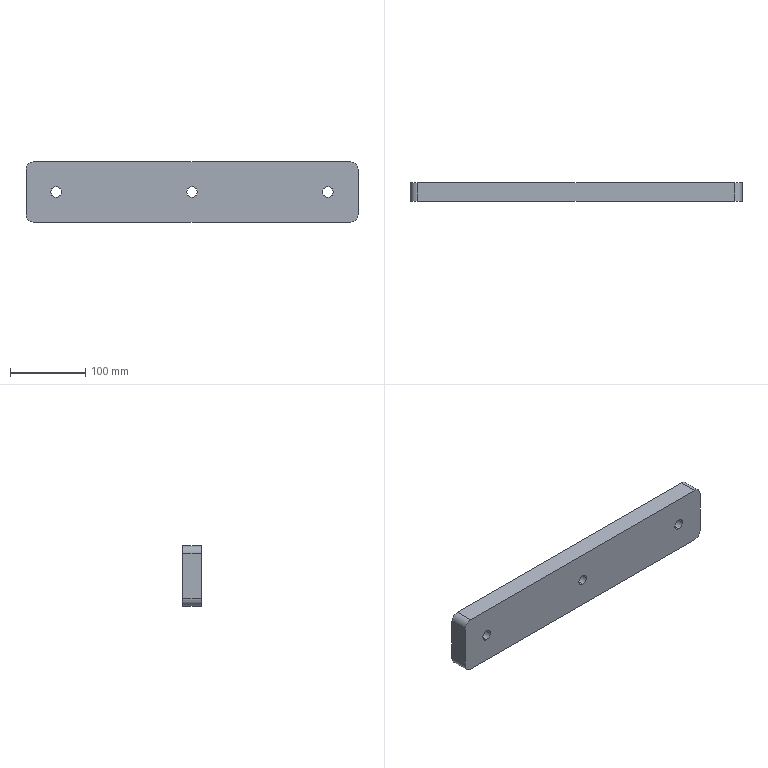Part | SolidWorks | features Fillet 1, FlatPattern 1, HoleWzd 1, LPattern 1, SMBaseFlange 1, SheetMetal 1 | 1 solid | 16 faces | box 440 x 25 x 80 mm | volume 866309 mm3 | cylinder 10 | plane 6 | commonest cylinder face diameters 14 x6 20 x4
STEP:
#1=CARTESIAN_POINT('',(180.,-25.,7.));
#2=VERTEX_POINT('',#1);
#3=CARTESIAN_POINT('',(180.,-25.,-7.));
#4=VERTEX_POINT('',#3);
#5=CARTESIAN_POINT('',(180.,-25.,0.));
#6=DIRECTION('',(0.,-1.,0.));
#7=DIRECTION('',(0.,0.,-1.));
#8=AXIS2_PLACEMENT_3D('',#5,#6,#7);
#9=CIRCLE('',#8,7.);
#10=EDGE_CURVE('',#2,#4,#9,.T.);
#11=ORIENTED_EDGE('',*,*,#10,.T.);
#12=CARTESIAN_POINT('',(180.,0.,-7.));
#13=VERTEX_POINT('',#12);
#14=CARTESIAN_POINT('',(180.,0.,-7.));
#15=DIRECTION('',(0.,1.,0.));
#16=VECTOR('',#15,1000.);
#17=LINE('',#14,#16);
#18=EDGE_CURVE('',#4,#13,#17,.T.);
#19=ORIENTED_EDGE('',*,*,#18,.T.);
#20=CARTESIAN_POINT('',(180.,0.,7.));
#21=VERTEX_POINT('',#20);
#22=CARTESIAN_POINT('',(180.,0.,0.));
#23=DIRECTION('',(0.,1.,0.));
#24=DIRECTION('',(0.,0.,1.));
#25=AXIS2_PLACEMENT_3D('',#22,#23,#24);
#26=CIRCLE('',#25,7.);
#27=EDGE_CURVE('',#13,#21,#26,.T.);
#28=ORIENTED_EDGE('',*,*,#27,.T.);
#29=CARTESIAN_POINT('',(180.,0.,7.));
#30=DIRECTION('',(0.,1.,0.));
#31=VECTOR('',#30,1000.);
#32=LINE('',#29,#31);
#33=EDGE_CURVE('',#2,#21,#32,.T.);
#34=ORIENTED_EDGE('',*,*,#33,.F.);
#35=EDGE_LOOP('',(#11,#19,#28,#34));
#36=FACE_OUTER_BOUND('',#35,.T.);
#37=CARTESIAN_POINT('',(180.,0.,0.));
#38=DIRECTION('',(0.,1.,0.));
#39=DIRECTION('',(0.,0.,1.));
#40=AXIS2_PLACEMENT_3D('',#37,#38,#39);
#41=CYLINDRICAL_SURFACE('',#40,7.);
#42=ADVANCED_FACE('',(#36),#41,.F.);
#43=CARTESIAN_POINT('',(-180.,-25.,7.));
#44=VERTEX_POINT('',#43);
#45=CARTESIAN_POINT('',(-180.,-25.,-7.));
#46=VERTEX_POINT('',#45);
#47=CARTESIAN_POINT('',(-180.,-25.,0.));
#48=DIRECTION('',(0.,-1.,0.));
#49=DIRECTION('',(0.,0.,-1.));
#50=AXIS2_PLACEMENT_3D('',#47,#48,#49);
#51=CIRCLE('',#50,7.);
#52=EDGE_CURVE('',#44,#46,#51,.T.);
#53=ORIENTED_EDGE('',*,*,#52,.T.);
#54=CARTESIAN_POINT('',(-180.,0.,-7.));
#55=VERTEX_POINT('',#54);
#56=CARTESIAN_POINT('',(-180.,0.,-7.));
#57=DIRECTION('',(0.,1.,0.));
#58=VECTOR('',#57,1000.);
#59=LINE('',#56,#58);
#60=EDGE_CURVE('',#46,#55,#59,.T.);
#61=ORIENTED_EDGE('',*,*,#60,.T.);
#62=CARTESIAN_POINT('',(-180.,0.,7.));
#63=VERTEX_POINT('',#62);
#64=CARTESIAN_POINT('',(-180.,0.,0.));
#65=DIRECTION('',(0.,1.,0.));
#66=DIRECTION('',(0.,0.,1.));
#67=AXIS2_PLACEMENT_3D('',#64,#65,#66);
#68=CIRCLE('',#67,7.);
#69=EDGE_CURVE('',#55,#63,#68,.T.);
#70=ORIENTED_EDGE('',*,*,#69,.T.);
#71=CARTESIAN_POINT('',(-180.,0.,7.));
#72=DIRECTION('',(0.,1.,0.));
#73=VECTOR('',#72,1000.);
#74=LINE('',#71,#73);
#75=EDGE_CURVE('',#44,#63,#74,.T.);
#76=ORIENTED_EDGE('',*,*,#75,.F.);
#77=EDGE_LOOP('',(#53,#61,#70,#76));
#78=FACE_OUTER_BOUND('',#77,.T.);
#79=CARTESIAN_POINT('',(-180.,0.,0.));
#80=DIRECTION('',(0.,1.,0.));
#81=DIRECTION('',(0.,0.,1.));
#82=AXIS2_PLACEMENT_3D('',#79,#80,#81);
#83=CYLINDRICAL_SURFACE('',#82,7.);
#84=ADVANCED_FACE('',(#78),#83,.F.);
#85=CARTESIAN_POINT('',(0.,-25.,7.));
#86=VERTEX_POINT('',#85);
#87=CARTESIAN_POINT('',(0.,-25.,-7.));
#88=VERTEX_POINT('',#87);
#89=CARTESIAN_POINT('',(0.,-25.,0.));
#90=DIRECTION('',(0.,-1.,0.));
#91=DIRECTION('',(0.,0.,-1.));
#92=AXIS2_PLACEMENT_3D('',#89,#90,#91);
#93=CIRCLE('',#92,7.);
#94=EDGE_CURVE('',#86,#88,#93,.T.);
#95=ORIENTED_EDGE('',*,*,#94,.T.);
#96=CARTESIAN_POINT('',(0.,0.,-7.));
#97=VERTEX_POINT('',#96);
#98=CARTESIAN_POINT('',(0.,0.,-7.));
#99=DIRECTION('',(0.,1.,0.));
#100=VECTOR('',#99,1000.);
#101=LINE('',#98,#100);
#102=EDGE_CURVE('',#88,#97,#101,.T.);
#103=ORIENTED_EDGE('',*,*,#102,.T.);
#104=CARTESIAN_POINT('',(0.,0.,7.));
#105=VERTEX_POINT('',#104);
#106=CARTESIAN_POINT('',(0.,0.,0.));
#107=DIRECTION('',(0.,1.,0.));
#108=DIRECTION('',(0.,0.,1.));
#109=AXIS2_PLACEMENT_3D('',#106,#107,#108);
#110=CIRCLE('',#109,7.);
#111=EDGE_CURVE('',#97,#105,#110,.T.);
#112=ORIENTED_EDGE('',*,*,#111,.T.);
#113=CARTESIAN_POINT('',(0.,0.,7.));
#114=DIRECTION('',(0.,1.,0.));
#115=VECTOR('',#114,1000.);
#116=LINE('',#113,#115);
#117=EDGE_CURVE('',#86,#105,#116,.T.);
#118=ORIENTED_EDGE('',*,*,#117,.F.);
#119=EDGE_LOOP('',(#95,#103,#112,#118));
#120=FACE_OUTER_BOUND('',#119,.T.);
#121=CARTESIAN_POINT('',(0.,0.,0.));
#122=DIRECTION('',(0.,1.,0.));
#123=DIRECTION('',(0.,0.,1.));
#124=AXIS2_PLACEMENT_3D('',#121,#122,#123);
#125=CYLINDRICAL_SURFACE('',#124,7.);
#126=ADVANCED_FACE('',(#120),#125,.F.);
#127=CARTESIAN_POINT('',(220.,0.,30.));
#128=VERTEX_POINT('',#127);
#129=CARTESIAN_POINT('',(220.,0.,-30.));
#130=VERTEX_POINT('',#129);
#131=CARTESIAN_POINT('',(220.,0.,40.));
#132=DIRECTION('',(0.,0.,-1.));
#133=VECTOR('',#132,1000.);
#134=LINE('',#131,#133);
#135=EDGE_CURVE('',#128,#130,#134,.T.);
#136=ORIENTED_EDGE('',*,*,#135,.F.);
#137=CARTESIAN_POINT('',(220.,-25.,30.));
#138=VERTEX_POINT('',#137);
#139=CARTESIAN_POINT('',(220.,-25.,30.));
#140=DIRECTION('',(0.,-1.,0.));
#141=VECTOR('',#140,1000.);
#142=LINE('',#139,#141);
#143=EDGE_CURVE('',#128,#138,#142,.T.);
#144=ORIENTED_EDGE('',*,*,#143,.T.);
#145=CARTESIAN_POINT('',(220.,-25.,-30.));
#146=VERTEX_POINT('',#145);
#147=CARTESIAN_POINT('',(220.,-25.,40.));
#148=DIRECTION('',(0.,0.,-1.));
#149=VECTOR('',#148,1000.);
#150=LINE('',#147,#149);
#151=EDGE_CURVE('',#138,#146,#150,.T.);
#152=ORIENTED_EDGE('',*,*,#151,.T.);
#153=CARTESIAN_POINT('',(220.,-25.,-30.));
#154=DIRECTION('',(0.,1.,0.));
#155=VECTOR('',#154,1000.);
#156=LINE('',#153,#155);
#157=EDGE_CURVE('',#146,#130,#156,.T.);
#158=ORIENTED_EDGE('',*,*,#157,.T.);
#159=EDGE_LOOP('',(#136,#144,#152,#158));
#160=FACE_OUTER_BOUND('',#159,.T.);
#161=CARTESIAN_POINT('',(220.,-25.,40.));
#162=DIRECTION('',(1.,0.,0.));
#163=DIRECTION('',(0.,0.,-1.));
#164=AXIS2_PLACEMENT_3D('',#161,#162,#163);
#165=PLANE('',#164);
#166=ADVANCED_FACE('',(#160),#165,.T.);
#167=CARTESIAN_POINT('',(-210.,-25.,40.));
#168=VERTEX_POINT('',#167);
#169=CARTESIAN_POINT('',(210.,-25.,40.));
#170=VERTEX_POINT('',#169);
#171=CARTESIAN_POINT('',(-220.,-25.,40.));
#172=DIRECTION('',(1.,0.,0.));
#173=VECTOR('',#172,1000.);
#174=LINE('',#171,#173);
#175=EDGE_CURVE('',#168,#170,#174,.T.);
#176=ORIENTED_EDGE('',*,*,#175,.T.);
#177=CARTESIAN_POINT('',(210.,0.,40.));
#178=VERTEX_POINT('',#177);
#179=CARTESIAN_POINT('',(210.,-25.,40.));
#180=DIRECTION('',(0.,1.,0.));
#181=VECTOR('',#180,1000.);
#182=LINE('',#179,#181);
#183=EDGE_CURVE('',#170,#178,#182,.T.);
#184=ORIENTED_EDGE('',*,*,#183,.T.);
#185=CARTESIAN_POINT('',(-210.,0.,40.));
#186=VERTEX_POINT('',#185);
#187=CARTESIAN_POINT('',(-220.,0.,40.));
#188=DIRECTION('',(1.,0.,0.));
#189=VECTOR('',#188,1000.);
#190=LINE('',#187,#189);
#191=EDGE_CURVE('',#186,#178,#190,.T.);
#192=ORIENTED_EDGE('',*,*,#191,.F.);
#193=CARTESIAN_POINT('',(-210.,-25.,40.));
#194=DIRECTION('',(0.,-1.,0.));
#195=VECTOR('',#194,1000.);
#196=LINE('',#193,#195);
#197=EDGE_CURVE('',#186,#168,#196,.T.);
#198=ORIENTED_EDGE('',*,*,#197,.T.);
#199=EDGE_LOOP('',(#176,#184,#192,#198));
#200=FACE_OUTER_BOUND('',#199,.T.);
#201=CARTESIAN_POINT('',(-220.,-25.,40.));
#202=DIRECTION('',(0.,0.,1.));
#203=DIRECTION('',(1.,0.,0.));
#204=AXIS2_PLACEMENT_3D('',#201,#202,#203);
#205=PLANE('',#204);
#206=ADVANCED_FACE('',(#200),#205,.T.);
#207=CARTESIAN_POINT('',(-220.,-25.,-30.));
#208=VERTEX_POINT('',#207);
#209=CARTESIAN_POINT('',(-220.,-25.,30.));
#210=VERTEX_POINT('',#209);
#211=CARTESIAN_POINT('',(-220.,-25.,40.));
#212=DIRECTION('',(0.,0.,1.));
#213=VECTOR('',#212,1000.);
#214=LINE('',#211,#213);
#215=EDGE_CURVE('',#208,#210,#214,.T.);
#216=ORIENTED_EDGE('',*,*,#215,.T.);
#217=CARTESIAN_POINT('',(-220.,0.,30.));
#218=VERTEX_POINT('',#217);
#219=CARTESIAN_POINT('',(-220.,-25.,30.));
#220=DIRECTION('',(0.,1.,0.));
#221=VECTOR('',#220,1000.);
#222=LINE('',#219,#221);
#223=EDGE_CURVE('',#210,#218,#222,.T.);
#224=ORIENTED_EDGE('',*,*,#223,.T.);
#225=CARTESIAN_POINT('',(-220.,0.,-30.));
#226=VERTEX_POINT('',#225);
#227=CARTESIAN_POINT('',(-220.,0.,40.));
#228=DIRECTION('',(0.,0.,1.));
#229=VECTOR('',#228,1000.);
#230=LINE('',#227,#229);
#231=EDGE_CURVE('',#226,#218,#230,.T.);
#232=ORIENTED_EDGE('',*,*,#231,.F.);
#233=CARTESIAN_POINT('',(-220.,-25.,-30.));
#234=DIRECTION('',(0.,-1.,0.));
#235=VECTOR('',#234,1000.);
#236=LINE('',#233,#235);
#237=EDGE_CURVE('',#226,#208,#236,.T.);
#238=ORIENTED_EDGE('',*,*,#237,.T.);
#239=EDGE_LOOP('',(#216,#224,#232,#238));
#240=FACE_OUTER_BOUND('',#239,.T.);
#241=CARTESIAN_POINT('',(-220.,-25.,40.));
#242=DIRECTION('',(-1.,0.,0.));
#243=DIRECTION('',(0.,0.,1.));
#244=AXIS2_PLACEMENT_3D('',#241,#242,#243);
#245=PLANE('',#244);
#246=ADVANCED_FACE('',(#240),#245,.T.);
#247=CARTESIAN_POINT('',(210.,0.,-40.));
#248=VERTEX_POINT('',#247);
#249=CARTESIAN_POINT('',(-210.,0.,-40.));
#250=VERTEX_POINT('',#249);
#251=CARTESIAN_POINT('',(-220.,0.,-40.));
#252=DIRECTION('',(-1.,0.,0.));
#253=VECTOR('',#252,1000.);
#254=LINE('',#251,#253);
#255=EDGE_CURVE('',#248,#250,#254,.T.);
#256=ORIENTED_EDGE('',*,*,#255,.F.);
#257=CARTESIAN_POINT('',(210.,-25.,-40.));
#258=VERTEX_POINT('',#257);
#259=CARTESIAN_POINT('',(210.,-25.,-40.));
#260=DIRECTION('',(0.,-1.,0.));
#261=VECTOR('',#260,1000.);
#262=LINE('',#259,#261);
#263=EDGE_CURVE('',#248,#258,#262,.T.);
#264=ORIENTED_EDGE('',*,*,#263,.T.);
#265=CARTESIAN_POINT('',(-210.,-25.,-40.));
#266=VERTEX_POINT('',#265);
#267=CARTESIAN_POINT('',(-220.,-25.,-40.));
#268=DIRECTION('',(-1.,0.,0.));
#269=VECTOR('',#268,1000.);
#270=LINE('',#267,#269);
#271=EDGE_CURVE('',#258,#266,#270,.T.);
#272=ORIENTED_EDGE('',*,*,#271,.T.);
#273=CARTESIAN_POINT('',(-210.,-25.,-40.));
#274=DIRECTION('',(0.,1.,0.));
#275=VECTOR('',#274,1000.);
#276=LINE('',#273,#275);
#277=EDGE_CURVE('',#266,#250,#276,.T.);
#278=ORIENTED_EDGE('',*,*,#277,.T.);
#279=EDGE_LOOP('',(#256,#264,#272,#278));
#280=FACE_OUTER_BOUND('',#279,.T.);
#281=CARTESIAN_POINT('',(-220.,-25.,-40.));
#282=DIRECTION('',(0.,0.,-1.));
#283=DIRECTION('',(-1.,0.,0.));
#284=AXIS2_PLACEMENT_3D('',#281,#282,#283);
#285=PLANE('',#284);
#286=ADVANCED_FACE('',(#280),#285,.T.);
#287=ORIENTED_EDGE('',*,*,#10,.F.);
#288=CARTESIAN_POINT('',(180.,-25.,0.));
#289=DIRECTION('',(0.,-1.,0.));
#290=DIRECTION('',(0.,0.,-1.));
#291=AXIS2_PLACEMENT_3D('',#288,#289,#290);
#292=CIRCLE('',#291,7.);
#293=EDGE_CURVE('',#4,#2,#292,.T.);
#294=ORIENTED_EDGE('',*,*,#293,.F.);
#295=EDGE_LOOP('',(#287,#294));
#296=FACE_BOUND('',#295,.T.);
#297=ORIENTED_EDGE('',*,*,#52,.F.);
#298=CARTESIAN_POINT('',(-180.,-25.,0.));
#299=DIRECTION('',(0.,-1.,0.));
#300=DIRECTION('',(0.,0.,-1.));
#301=AXIS2_PLACEMENT_3D('',#298,#299,#300);
#302=CIRCLE('',#301,7.);
#303=EDGE_CURVE('',#46,#44,#302,.T.);
#304=ORIENTED_EDGE('',*,*,#303,.F.);
#305=EDGE_LOOP('',(#297,#304));
#306=FACE_BOUND('',#305,.T.);
#307=ORIENTED_EDGE('',*,*,#94,.F.);
#308=CARTESIAN_POINT('',(0.,-25.,0.));
#309=DIRECTION('',(0.,-1.,0.));
#310=DIRECTION('',(0.,0.,-1.));
#311=AXIS2_PLACEMENT_3D('',#308,#309,#310);
#312=CIRCLE('',#311,7.);
#313=EDGE_CURVE('',#88,#86,#312,.T.);
#314=ORIENTED_EDGE('',*,*,#313,.F.);
#315=EDGE_LOOP('',(#307,#314));
#316=FACE_BOUND('',#315,.T.);
#317=ORIENTED_EDGE('',*,*,#151,.F.);
#318=CARTESIAN_POINT('',(210.,-25.,30.));
#319=DIRECTION('',(0.,-1.,0.));
#320=DIRECTION('',(0.,0.,-1.));
#321=AXIS2_PLACEMENT_3D('',#318,#319,#320);
#322=CIRCLE('',#321,10.);
#323=EDGE_CURVE('',#138,#170,#322,.T.);
#324=ORIENTED_EDGE('',*,*,#323,.T.);
#325=ORIENTED_EDGE('',*,*,#175,.F.);
#326=CARTESIAN_POINT('',(-210.,-25.,30.));
#327=DIRECTION('',(0.,-1.,0.));
#328=DIRECTION('',(0.,0.,-1.));
#329=AXIS2_PLACEMENT_3D('',#326,#327,#328);
#330=CIRCLE('',#329,10.);
#331=EDGE_CURVE('',#168,#210,#330,.T.);
#332=ORIENTED_EDGE('',*,*,#331,.T.);
#333=ORIENTED_EDGE('',*,*,#215,.F.);
#334=CARTESIAN_POINT('',(-210.,-25.,-30.));
#335=DIRECTION('',(0.,-1.,0.));
#336=DIRECTION('',(0.,0.,-1.));
#337=AXIS2_PLACEMENT_3D('',#334,#335,#336);
#338=CIRCLE('',#337,10.);
#339=EDGE_CURVE('',#208,#266,#338,.T.);
#340=ORIENTED_EDGE('',*,*,#339,.T.);
#341=ORIENTED_EDGE('',*,*,#271,.F.);
#342=CARTESIAN_POINT('',(210.,-25.,-30.));
#343=DIRECTION('',(0.,-1.,0.));
#344=DIRECTION('',(0.,0.,-1.));
#345=AXIS2_PLACEMENT_3D('',#342,#343,#344);
#346=CIRCLE('',#345,10.);
#347=EDGE_CURVE('',#258,#146,#346,.T.);
#348=ORIENTED_EDGE('',*,*,#347,.T.);
#349=EDGE_LOOP('',(#317,#324,#325,#332,#333,#340,#341,#348));
#350=FACE_OUTER_BOUND('',#349,.T.);
#351=CARTESIAN_POINT('',(0.,-25.,0.));
#352=DIRECTION('',(0.,-1.,0.));
#353=DIRECTION('',(0.,0.,-1.));
#354=AXIS2_PLACEMENT_3D('',#351,#352,#353);
#355=PLANE('',#354);
#356=ADVANCED_FACE('',(#296,#306,#316,#350),#355,.T.);
#357=CARTESIAN_POINT('',(180.,0.,0.));
#358=DIRECTION('',(0.,1.,0.));
#359=DIRECTION('',(0.,0.,1.));
#360=AXIS2_PLACEMENT_3D('',#357,#358,#359);
#361=CIRCLE('',#360,7.);
#362=EDGE_CURVE('',#21,#13,#361,.T.);
#363=ORIENTED_EDGE('',*,*,#362,.F.);
#364=ORIENTED_EDGE('',*,*,#27,.F.);
#365=EDGE_LOOP('',(#363,#364));
#366=FACE_BOUND('',#365,.T.);
#367=CARTESIAN_POINT('',(-180.,0.,0.));
#368=DIRECTION('',(0.,1.,0.));
#369=DIRECTION('',(0.,0.,1.));
#370=AXIS2_PLACEMENT_3D('',#367,#368,#369);
#371=CIRCLE('',#370,7.);
#372=EDGE_CURVE('',#63,#55,#371,.T.);
#373=ORIENTED_EDGE('',*,*,#372,.F.);
#374=ORIENTED_EDGE('',*,*,#69,.F.);
#375=EDGE_LOOP('',(#373,#374));
#376=FACE_BOUND('',#375,.T.);
#377=CARTESIAN_POINT('',(0.,0.,0.));
#378=DIRECTION('',(0.,1.,0.));
#379=DIRECTION('',(0.,0.,1.));
#380=AXIS2_PLACEMENT_3D('',#377,#378,#379);
#381=CIRCLE('',#380,7.);
#382=EDGE_CURVE('',#105,#97,#381,.T.);
#383=ORIENTED_EDGE('',*,*,#382,.F.);
#384=ORIENTED_EDGE('',*,*,#111,.F.);
#385=EDGE_LOOP('',(#383,#384));
#386=FACE_BOUND('',#385,.T.);
#387=ORIENTED_EDGE('',*,*,#191,.T.);
#388=CARTESIAN_POINT('',(210.,0.,30.));
#389=DIRECTION('',(0.,1.,0.));
#390=DIRECTION('',(0.,0.,-1.));
#391=AXIS2_PLACEMENT_3D('',#388,#389,#390);
#392=CIRCLE('',#391,10.);
#393=EDGE_CURVE('',#178,#128,#392,.T.);
#394=ORIENTED_EDGE('',*,*,#393,.T.);
#395=ORIENTED_EDGE('',*,*,#135,.T.);
#396=CARTESIAN_POINT('',(210.,0.,-30.));
#397=DIRECTION('',(0.,1.,0.));
#398=DIRECTION('',(0.,0.,-1.));
#399=AXIS2_PLACEMENT_3D('',#396,#397,#398);
#400=CIRCLE('',#399,10.);
#401=EDGE_CURVE('',#130,#248,#400,.T.);
#402=ORIENTED_EDGE('',*,*,#401,.T.);
#403=ORIENTED_EDGE('',*,*,#255,.T.);
#404=CARTESIAN_POINT('',(-210.,0.,-30.));
#405=DIRECTION('',(0.,1.,0.));
#406=DIRECTION('',(0.,0.,-1.));
#407=AXIS2_PLACEMENT_3D('',#404,#405,#406);
#408=CIRCLE('',#407,10.);
#409=EDGE_CURVE('',#250,#226,#408,.T.);
#410=ORIENTED_EDGE('',*,*,#409,.T.);
#411=ORIENTED_EDGE('',*,*,#231,.T.);
#412=CARTESIAN_POINT('',(-210.,0.,30.));
#413=DIRECTION('',(0.,1.,0.));
#414=DIRECTION('',(0.,0.,-1.));
#415=AXIS2_PLACEMENT_3D('',#412,#413,#414);
#416=CIRCLE('',#415,10.);
#417=EDGE_CURVE('',#218,#186,#416,.T.);
#418=ORIENTED_EDGE('',*,*,#417,.T.);
#419=EDGE_LOOP('',(#387,#394,#395,#402,#403,#410,#411,#418));
#420=FACE_OUTER_BOUND('',#419,.T.);
#421=CARTESIAN_POINT('',(0.,0.,0.));
#422=DIRECTION('',(0.,-1.,0.));
#423=DIRECTION('',(0.,0.,-1.));
#424=AXIS2_PLACEMENT_3D('',#421,#422,#423);
#425=PLANE('',#424);
#426=ADVANCED_FACE('',(#366,#376,#386,#420),#425,.F.);
#427=ORIENTED_EDGE('',*,*,#102,.F.);
#428=ORIENTED_EDGE('',*,*,#313,.T.);
#429=ORIENTED_EDGE('',*,*,#117,.T.);
#430=ORIENTED_EDGE('',*,*,#382,.T.);
#431=EDGE_LOOP('',(#427,#428,#429,#430));
#432=FACE_OUTER_BOUND('',#431,.T.);
#433=CARTESIAN_POINT('',(0.,0.,0.));
#434=DIRECTION('',(0.,1.,0.));
#435=DIRECTION('',(0.,0.,1.));
#436=AXIS2_PLACEMENT_3D('',#433,#434,#435);
#437=CYLINDRICAL_SURFACE('',#436,7.);
#438=ADVANCED_FACE('',(#432),#437,.F.);
#439=ORIENTED_EDGE('',*,*,#60,.F.);
#440=ORIENTED_EDGE('',*,*,#303,.T.);
#441=ORIENTED_EDGE('',*,*,#75,.T.);
#442=ORIENTED_EDGE('',*,*,#372,.T.);
#443=EDGE_LOOP('',(#439,#440,#441,#442));
#444=FACE_OUTER_BOUND('',#443,.T.);
#445=CARTESIAN_POINT('',(-180.,0.,0.));
#446=DIRECTION('',(0.,1.,0.));
#447=DIRECTION('',(0.,0.,1.));
#448=AXIS2_PLACEMENT_3D('',#445,#446,#447);
#449=CYLINDRICAL_SURFACE('',#448,7.);
#450=ADVANCED_FACE('',(#444),#449,.F.);
#451=ORIENTED_EDGE('',*,*,#18,.F.);
#452=ORIENTED_EDGE('',*,*,#293,.T.);
#453=ORIENTED_EDGE('',*,*,#33,.T.);
#454=ORIENTED_EDGE('',*,*,#362,.T.);
#455=EDGE_LOOP('',(#451,#452,#453,#454));
#456=FACE_OUTER_BOUND('',#455,.T.);
#457=CARTESIAN_POINT('',(180.,0.,0.));
#458=DIRECTION('',(0.,1.,0.));
#459=DIRECTION('',(0.,0.,1.));
#460=AXIS2_PLACEMENT_3D('',#457,#458,#459);
#461=CYLINDRICAL_SURFACE('',#460,7.);
#462=ADVANCED_FACE('',(#456),#461,.F.);
#463=ORIENTED_EDGE('',*,*,#323,.F.);
#464=ORIENTED_EDGE('',*,*,#143,.F.);
#465=ORIENTED_EDGE('',*,*,#393,.F.);
#466=ORIENTED_EDGE('',*,*,#183,.F.);
#467=EDGE_LOOP('',(#463,#464,#465,#466));
#468=FACE_OUTER_BOUND('',#467,.T.);
#469=CARTESIAN_POINT('',(210.,-25.,30.));
#470=DIRECTION('',(0.,1.,0.));
#471=DIRECTION('',(0.,0.,1.));
#472=AXIS2_PLACEMENT_3D('',#469,#470,#471);
#473=CYLINDRICAL_SURFACE('',#472,10.);
#474=ADVANCED_FACE('',(#468),#473,.T.);
#475=ORIENTED_EDGE('',*,*,#347,.F.);
#476=ORIENTED_EDGE('',*,*,#263,.F.);
#477=ORIENTED_EDGE('',*,*,#401,.F.);
#478=ORIENTED_EDGE('',*,*,#157,.F.);
#479=EDGE_LOOP('',(#475,#476,#477,#478));
#480=FACE_OUTER_BOUND('',#479,.T.);
#481=CARTESIAN_POINT('',(210.,-25.,-30.));
#482=DIRECTION('',(0.,1.,0.));
#483=DIRECTION('',(0.,0.,1.));
#484=AXIS2_PLACEMENT_3D('',#481,#482,#483);
#485=CYLINDRICAL_SURFACE('',#484,10.);
#486=ADVANCED_FACE('',(#480),#485,.T.);
#487=ORIENTED_EDGE('',*,*,#331,.F.);
#488=ORIENTED_EDGE('',*,*,#197,.F.);
#489=ORIENTED_EDGE('',*,*,#417,.F.);
#490=ORIENTED_EDGE('',*,*,#223,.F.);
#491=EDGE_LOOP('',(#487,#488,#489,#490));
#492=FACE_OUTER_BOUND('',#491,.T.);
#493=CARTESIAN_POINT('',(-210.,-25.,30.));
#494=DIRECTION('',(0.,1.,0.));
#495=DIRECTION('',(0.,0.,1.));
#496=AXIS2_PLACEMENT_3D('',#493,#494,#495);
#497=CYLINDRICAL_SURFACE('',#496,10.);
#498=ADVANCED_FACE('',(#492),#497,.T.);
#499=ORIENTED_EDGE('',*,*,#339,.F.);
#500=ORIENTED_EDGE('',*,*,#237,.F.);
#501=ORIENTED_EDGE('',*,*,#409,.F.);
#502=ORIENTED_EDGE('',*,*,#277,.F.);
#503=EDGE_LOOP('',(#499,#500,#501,#502));
#504=FACE_OUTER_BOUND('',#503,.T.);
#505=CARTESIAN_POINT('',(-210.,-25.,-30.));
#506=DIRECTION('',(0.,1.,0.));
#507=DIRECTION('',(0.,0.,1.));
#508=AXIS2_PLACEMENT_3D('',#505,#506,#507);
#509=CYLINDRICAL_SURFACE('',#508,10.);
#510=ADVANCED_FACE('',(#504),#509,.T.);
#511=CLOSED_SHELL('',(#42,#84,#126,#166,#206,#246,#286,#356,#426,#438,#450,#462,#474,#486,#498,#510));
#512=MANIFOLD_SOLID_BREP('',#511);
#513=CARTESIAN_POINT('',(0.,0.,0.));
#514=DIRECTION('',(0.,0.,1.));
#515=DIRECTION('',(1.,0.,0.));
#516=AXIS2_PLACEMENT_3D('',#513,#514,#515);
#517=(LENGTH_UNIT()NAMED_UNIT(*)SI_UNIT(.MILLI.,.METRE.));
#518=UNCERTAINTY_MEASURE_WITH_UNIT(LENGTH_MEASURE(0.00001),#517,'','');
#519=(NAMED_UNIT(*)PLANE_ANGLE_UNIT()SI_UNIT($,.RADIAN.));
#520=(NAMED_UNIT(*)SI_UNIT($,.STERADIAN.)SOLID_ANGLE_UNIT());
#521=(GEOMETRIC_REPRESENTATION_CONTEXT(3)GLOBAL_UNCERTAINTY_ASSIGNED_CONTEXT((#518))GLOBAL_UNIT_ASSIGNED_CONTEXT((#517,#519,#520))REPRESENTATION_CONTEXT('',''));
#522=ADVANCED_BREP_SHAPE_REPRESENTATION('',(#512,#516),#521);